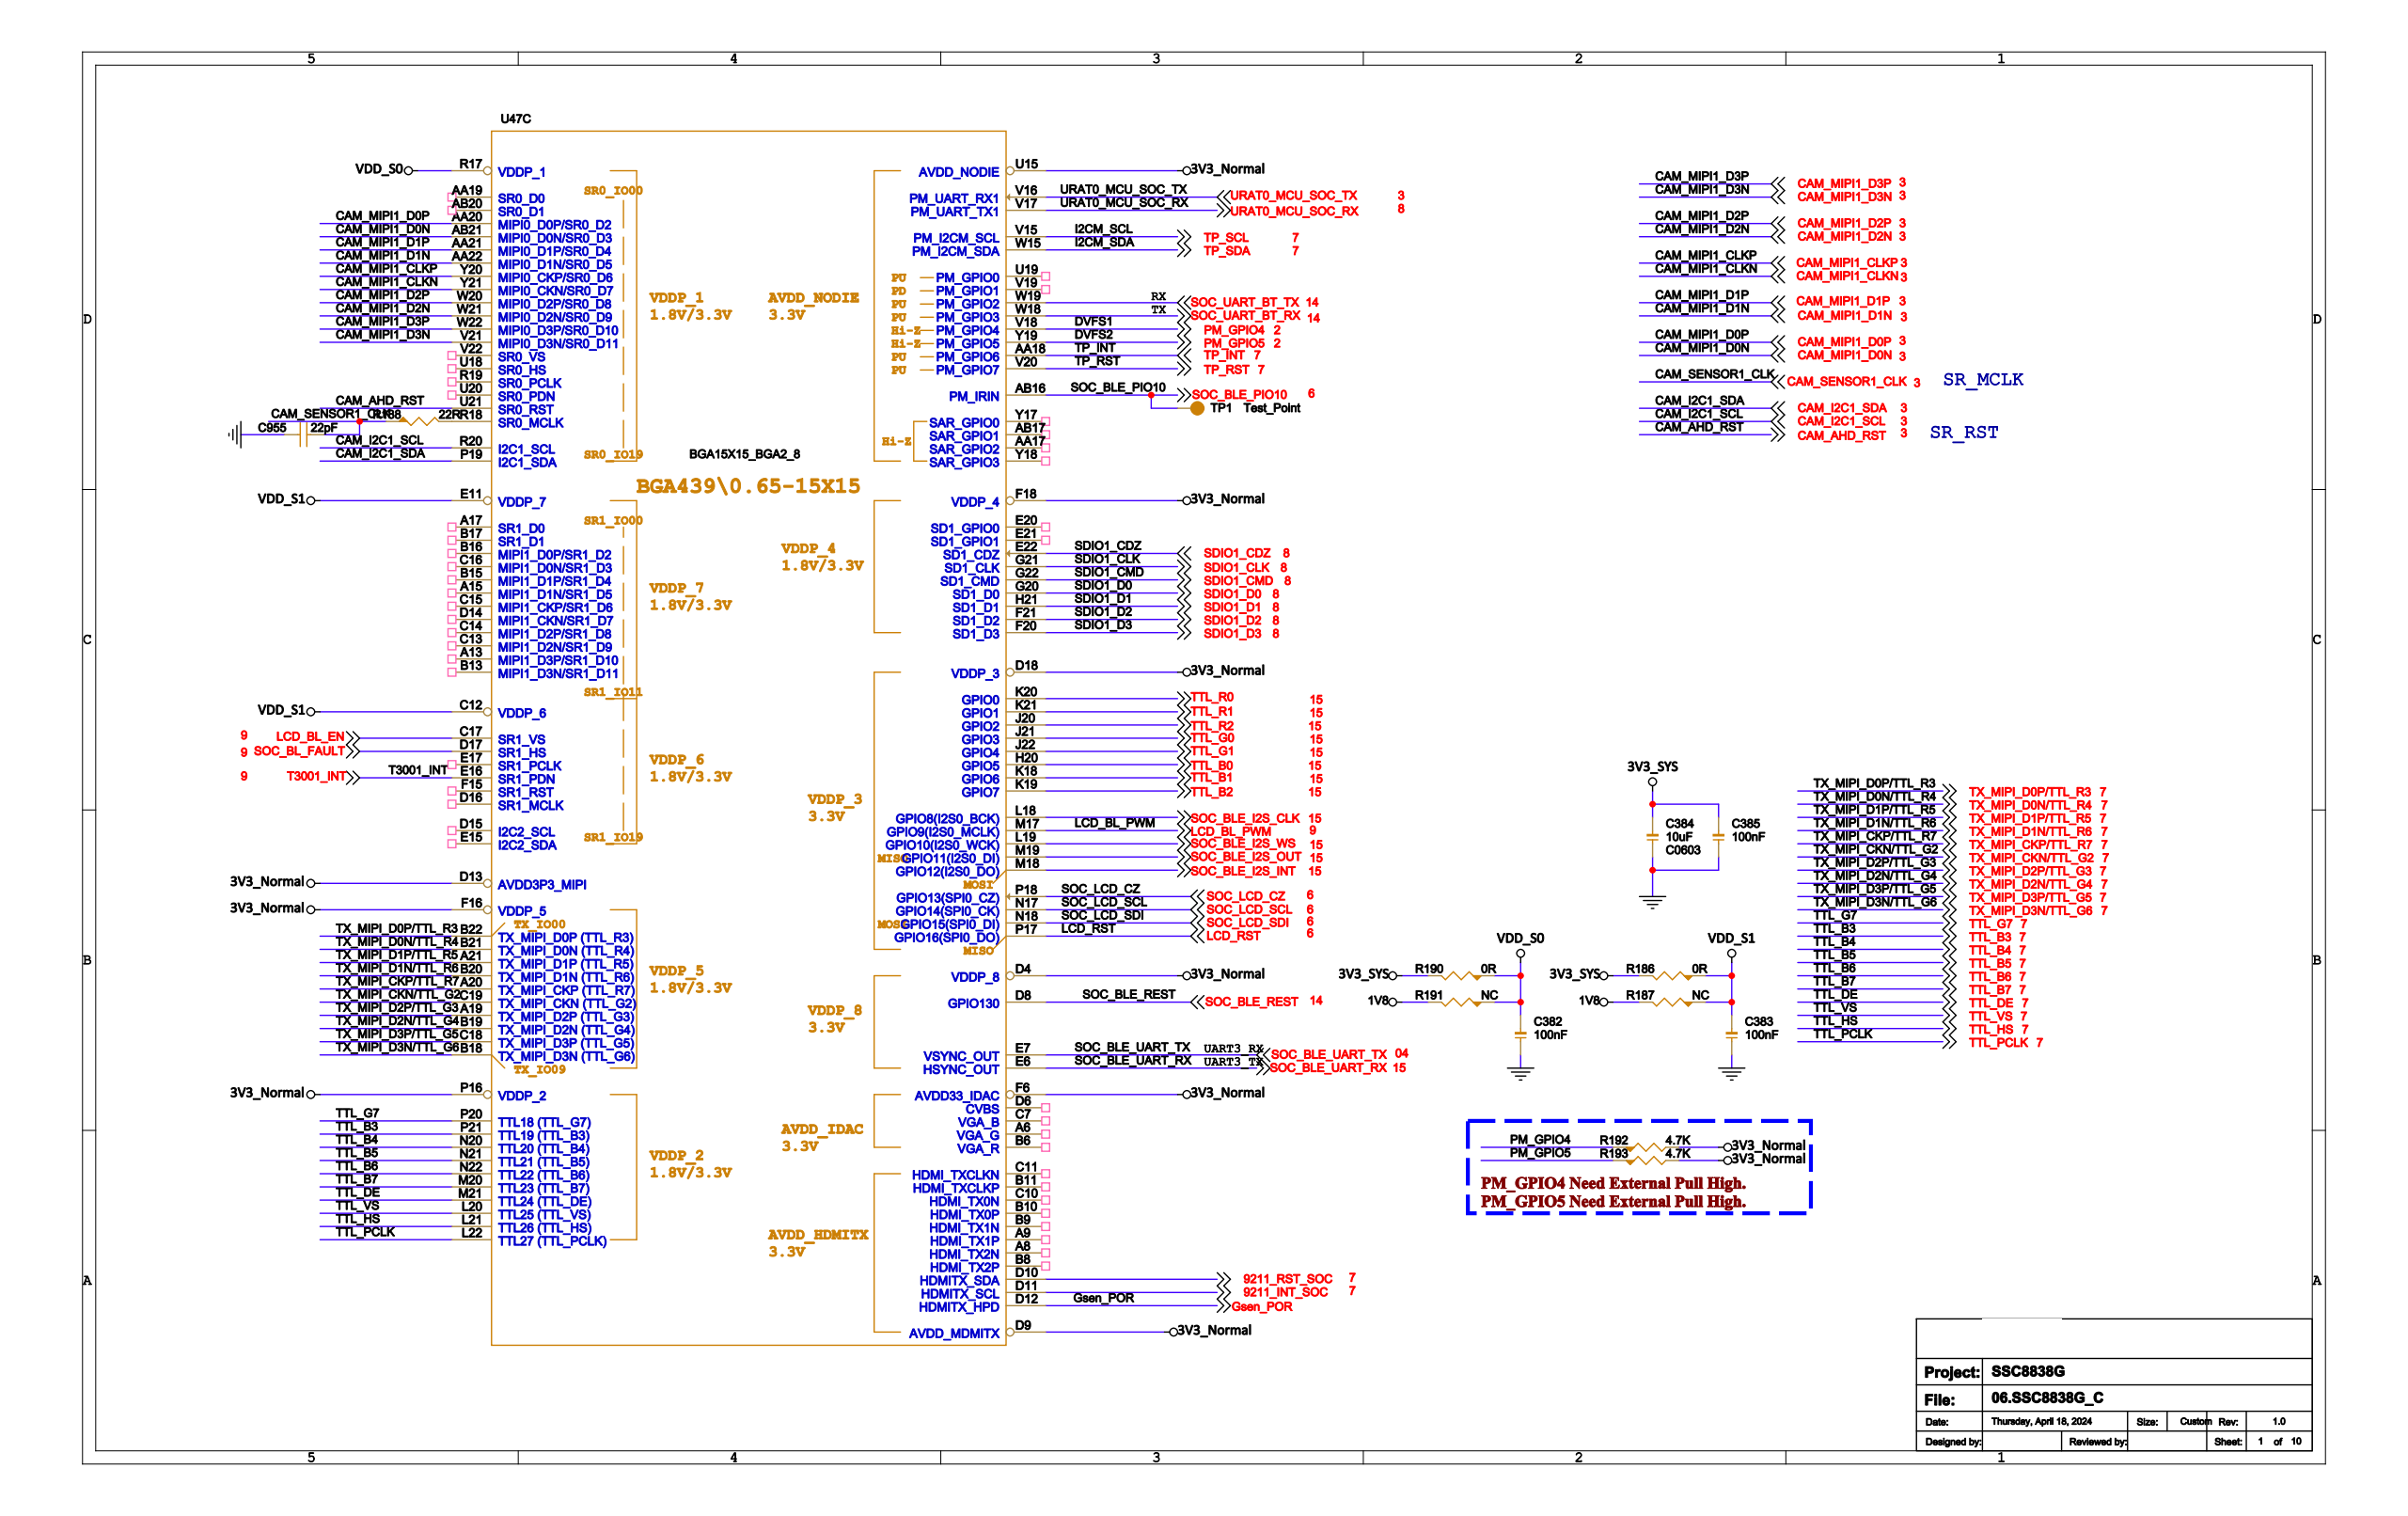Circuit board | Cadence Allegro | 958 parts | 601 nets | one sheet of the schematic
Parts on this sheet (reference | value | footprint):
C382 | 100nF | C0402
C383 | 100nF | C0402
C384 | 10uF | C0603
C385 | 100nF | C0402
C955 | 22pF | C0402
R186 | 0R | R0402
R187 | NC | R0402
R188 | 22R | R0402
R190 | 0R | R0402
R191 | NC | R0402
R192 | 4.7K | R0402
R193 | 4.7K | R0402
TP1 | Test_Point | TP_0R50
U21 | TP9963 | QFN40_5X5H0_8
U47 | BGA15X15_BGA2_8 | 8838G
Nets of these parts (net: part-pin ...):
GND: C382-2 C383-2 C384-2 C385-2 C955-1
3V3_NORMAL: C384-1 C385-1 R186-2 R190-2 R192-2 R193-2 U47-D4 U47-D9 U47-D13 U47-D18 U47-F6 U47-F16 U47-F18 U47-P16 U47-U15
LCD_RST: U47-P17
CAM_AHD_RST: U21-15 U47-U21
VDD_S0: C382-1 R190-1 R191-1 U47-R17
VDD_S1: C383-1 R186-1 R187-1 U47-C12 U47-E11
CAM_SENSOR1_CLK: C955-2 R188-1
TP_SDA: U47-W15
TP_SCL: U47-V15
TP_RST: U47-V20
TP_INT: U47-AA18
1V8: R187-2 R191-2
CAM_MIPI1_CLKP: U47-Y20
CAM_MIPI1_CLKN: U47-Y21
CAM_MIPI1_D0P: U47-AA20
CAM_MIPI1_D0N: U47-AB21
CAM_MIPI1_D1P: U47-AA21
CAM_MIPI1_D1N: U47-AA22
CAM_MIPI1_D3P: U47-W22
CAM_MIPI1_D3N: U47-V21
CAM_MIPI1_D2P: U47-W20
CAM_MIPI1_D2N: U47-W21
PM_GPIO5: R193-1 U47-Y19
PM_GPIO4: R192-1 U47-V18
CAM_I2C1_SCL: U47-R20
CAM_I2C1_SDA: U47-P19
SOC_UART_BT_RX: U47-W18
SOC_UART_BT_TX: U47-W19
N205324821: R188-2 U47-R18
SDIO1_D0: U47-G20
SDIO1_D1: U47-H21
SDIO1_D2: U47-F21
SDIO1_D3: U47-F20
SDIO1_CMD: U47-G22
SDIO1_CDZ: U47-E22
SDIO1_CLK: U47-G21
9211_RST_SOC: U47-D10
9211_INT_SOC: U47-D11
LCD_BL_EN: U47-C17
LCD_BL_PWM: U47-M17
SOC_BL_FAULT: U47-D17
TTL_DE: U47-M21
TTL_VS: U47-L20
TTL_HS: U47-L21
TTL_PCLK: U47-L22
SOC_LCD_CZ: U47-P18
TX_MIPI_D0P/TTL_R3: U47-B22
TX_MIPI_D0N/TTL_R4: U47-B21
TX_MIPI_D1N/TTL_R6: U47-B20
TX_MIPI_D1P/TTL_R5: U47-A21
TX_MIPI_D2P/TTL_G3: U47-A19
TX_MIPI_D2N/TTL_G4: U47-B19
TX_MIPI_CKP/TTL_R7: U47-A20
TX_MIPI_CKN/TTL_G2: U47-C19
TX_MIPI_D3N/TTL_G6: U47-B18
TX_MIPI_D3P/TTL_G5: U47-C18
TTL_R1: U47-K21
TTL_R0: U47-K20
TTL_R2: U47-J20
TTL_G0: U47-J21
TTL_G1: U47-J22
TTL_G7: U47-P20
TTL_B0: U47-H20
TTL_B1: U47-K18
TTL_B2: U47-K19
TTL_B3: U47-P21
TTL_B5: U47-N21
TTL_B4: U47-N20
TTL_B6: U47-N22
TTL_B7: U47-M20
SOC_LCD_SCL: U47-N17
SOC_LCD_SDI: U47-N18
SOC_BLE_PIO10: TP1-1 U47-AB16
SOC_BLE_REST: U47-D8
SOC_BLE_UART_TX: U47-E7
SOC_BLE_UART_RX: U47-E6
T3001_INT: U47-E16
URAT0_MCU_SOC_RX: U47-V17
URAT0_MCU_SOC_TX: U47-V16
SOC_BLE_I2S_WS: U47-L19
SOC_BLE_I2S_OUT: U47-M19
SOC_BLE_I2S_INT: U47-M18
SOC_BLE_I2S_CLK: U47-L18